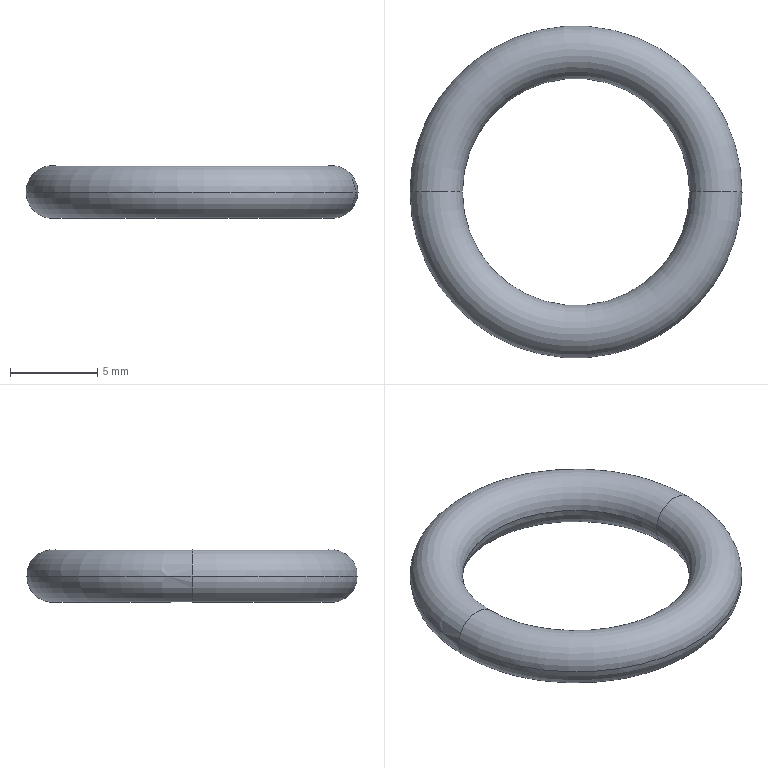Part | STEP file | MIFENGQUAN1 | 1 solid | 4 faces | box 19 x 19 x 3 mm | volume 355.306 mm3 | torus 4
STEP:
#1=CARTESIAN_POINT('',(0.,0.,0.));
#2=DIRECTION('',(0.,0.,1.));
#3=DIRECTION('',(1.,0.,0.));
#4=AXIS2_PLACEMENT_3D('',#1,#2,#3);
#5=CARTESIAN_POINT('',(-6.5,0.,0.));
#6=VERTEX_POINT('',#5);
#7=CARTESIAN_POINT('',(-9.5,0.,0.));
#8=VERTEX_POINT('',#7);
#9=CARTESIAN_POINT('',(-8.,0.,0.));
#10=DIRECTION('',(0.,1.,0.));
#11=DIRECTION('',(1.,0.,0.));
#12=AXIS2_PLACEMENT_3D('',#9,#10,#11);
#13=CIRCLE('',#12,1.5);
#14=EDGE_CURVE('',#6,#8,#13,.T.);
#15=ORIENTED_EDGE('',*,*,#14,.T.);
#16=CARTESIAN_POINT('',(9.5,0.,0.));
#17=VERTEX_POINT('',#16);
#18=CARTESIAN_POINT('',(0.,0.,0.));
#19=DIRECTION('',(0.,0.,1.));
#20=DIRECTION('',(-1.,0.,0.));
#21=AXIS2_PLACEMENT_3D('',#18,#19,#20);
#22=CIRCLE('',#21,9.5);
#23=EDGE_CURVE('',#8,#17,#22,.T.);
#24=ORIENTED_EDGE('',*,*,#23,.T.);
#25=CARTESIAN_POINT('',(6.5,0.,0.));
#26=VERTEX_POINT('',#25);
#27=CARTESIAN_POINT('',(8.,0.,0.));
#28=DIRECTION('',(0.,-1.,0.));
#29=DIRECTION('',(-1.,0.,0.));
#30=AXIS2_PLACEMENT_3D('',#27,#28,#29);
#31=CIRCLE('',#30,1.5);
#32=EDGE_CURVE('',#26,#17,#31,.T.);
#33=ORIENTED_EDGE('',*,*,#32,.F.);
#34=CARTESIAN_POINT('',(0.,0.,0.));
#35=DIRECTION('',(0.,0.,1.));
#36=DIRECTION('',(-1.,0.,0.));
#37=AXIS2_PLACEMENT_3D('',#34,#35,#36);
#38=CIRCLE('',#37,6.5);
#39=EDGE_CURVE('',#6,#26,#38,.T.);
#40=ORIENTED_EDGE('',*,*,#39,.F.);
#41=EDGE_LOOP('',(#15,#24,#33,#40));
#42=FACE_OUTER_BOUND('',#41,.F.);
#43=CARTESIAN_POINT('',(0.,0.,0.));
#44=DIRECTION('',(0.,0.,1.));
#45=DIRECTION('',(-1.,0.,0.));
#46=AXIS2_PLACEMENT_3D('',#43,#44,#45);
#47=TOROIDAL_SURFACE('',#46,8.,1.5);
#48=ADVANCED_FACE('',(#42),#47,.T.);
#49=ORIENTED_EDGE('',*,*,#14,.F.);
#50=CARTESIAN_POINT('',(0.,0.,0.));
#51=DIRECTION('',(0.,0.,-1.));
#52=DIRECTION('',(-1.,0.,0.));
#53=AXIS2_PLACEMENT_3D('',#50,#51,#52);
#54=CIRCLE('',#53,6.5);
#55=EDGE_CURVE('',#6,#26,#54,.T.);
#56=ORIENTED_EDGE('',*,*,#55,.T.);
#57=ORIENTED_EDGE('',*,*,#32,.T.);
#58=CARTESIAN_POINT('',(0.,0.,0.));
#59=DIRECTION('',(0.,0.,-1.));
#60=DIRECTION('',(-1.,0.,0.));
#61=AXIS2_PLACEMENT_3D('',#58,#59,#60);
#62=CIRCLE('',#61,9.5);
#63=EDGE_CURVE('',#8,#17,#62,.T.);
#64=ORIENTED_EDGE('',*,*,#63,.F.);
#65=EDGE_LOOP('',(#49,#56,#57,#64));
#66=FACE_OUTER_BOUND('',#65,.F.);
#67=CARTESIAN_POINT('',(0.,0.,0.));
#68=DIRECTION('',(0.,0.,1.));
#69=DIRECTION('',(-1.,0.,0.));
#70=AXIS2_PLACEMENT_3D('',#67,#68,#69);
#71=TOROIDAL_SURFACE('',#70,8.,1.5);
#72=ADVANCED_FACE('',(#66),#71,.T.);
#73=CARTESIAN_POINT('',(-8.,0.,0.));
#74=DIRECTION('',(0.,1.,0.));
#75=DIRECTION('',(-1.,0.,0.));
#76=AXIS2_PLACEMENT_3D('',#73,#74,#75);
#77=CIRCLE('',#76,1.5);
#78=EDGE_CURVE('',#8,#6,#77,.T.);
#79=ORIENTED_EDGE('',*,*,#78,.F.);
#80=ORIENTED_EDGE('',*,*,#63,.T.);
#81=CARTESIAN_POINT('',(8.,0.,0.));
#82=DIRECTION('',(0.,-1.,0.));
#83=DIRECTION('',(1.,0.,0.));
#84=AXIS2_PLACEMENT_3D('',#81,#82,#83);
#85=CIRCLE('',#84,1.5);
#86=EDGE_CURVE('',#17,#26,#85,.T.);
#87=ORIENTED_EDGE('',*,*,#86,.T.);
#88=ORIENTED_EDGE('',*,*,#55,.F.);
#89=EDGE_LOOP('',(#79,#80,#87,#88));
#90=FACE_OUTER_BOUND('',#89,.F.);
#91=CARTESIAN_POINT('',(0.,0.,0.));
#92=DIRECTION('',(0.,0.,1.));
#93=DIRECTION('',(-1.,0.,0.));
#94=AXIS2_PLACEMENT_3D('',#91,#92,#93);
#95=TOROIDAL_SURFACE('',#94,8.,1.5);
#96=ADVANCED_FACE('',(#90),#95,.T.);
#97=ORIENTED_EDGE('',*,*,#78,.T.);
#98=ORIENTED_EDGE('',*,*,#39,.T.);
#99=ORIENTED_EDGE('',*,*,#86,.F.);
#100=ORIENTED_EDGE('',*,*,#23,.F.);
#101=EDGE_LOOP('',(#97,#98,#99,#100));
#102=FACE_OUTER_BOUND('',#101,.F.);
#103=CARTESIAN_POINT('',(0.,0.,0.));
#104=DIRECTION('',(0.,0.,1.));
#105=DIRECTION('',(-1.,0.,0.));
#106=AXIS2_PLACEMENT_3D('',#103,#104,#105);
#107=TOROIDAL_SURFACE('',#106,8.,1.5);
#108=ADVANCED_FACE('',(#102),#107,.T.);
#109=CLOSED_SHELL('',(#48,#72,#96,#108));
#110=MANIFOLD_SOLID_BREP('',#109);
#111=(LENGTH_UNIT()NAMED_UNIT(*)SI_UNIT(.MILLI.,.METRE.));
#112=UNCERTAINTY_MEASURE_WITH_UNIT(LENGTH_MEASURE(0.002704),#111,'','');
#113=(NAMED_UNIT(*)PLANE_ANGLE_UNIT()SI_UNIT($,.RADIAN.));
#114=PLANE_ANGLE_MEASURE_WITH_UNIT(PLANE_ANGLE_MEASURE(0.01745),#113);
#115=(CONVERSION_BASED_UNIT('DEGREE',#114)NAMED_UNIT(*)PLANE_ANGLE_UNIT());
#116=(NAMED_UNIT(*)SI_UNIT($,.STERADIAN.)SOLID_ANGLE_UNIT());
#117=(GEOMETRIC_REPRESENTATION_CONTEXT(3)GLOBAL_UNCERTAINTY_ASSIGNED_CONTEXT((#112))GLOBAL_UNIT_ASSIGNED_CONTEXT((#111,#115,#116))REPRESENTATION_CONTEXT('',''));
#118=ADVANCED_BREP_SHAPE_REPRESENTATION('',(#4,#110),#117);